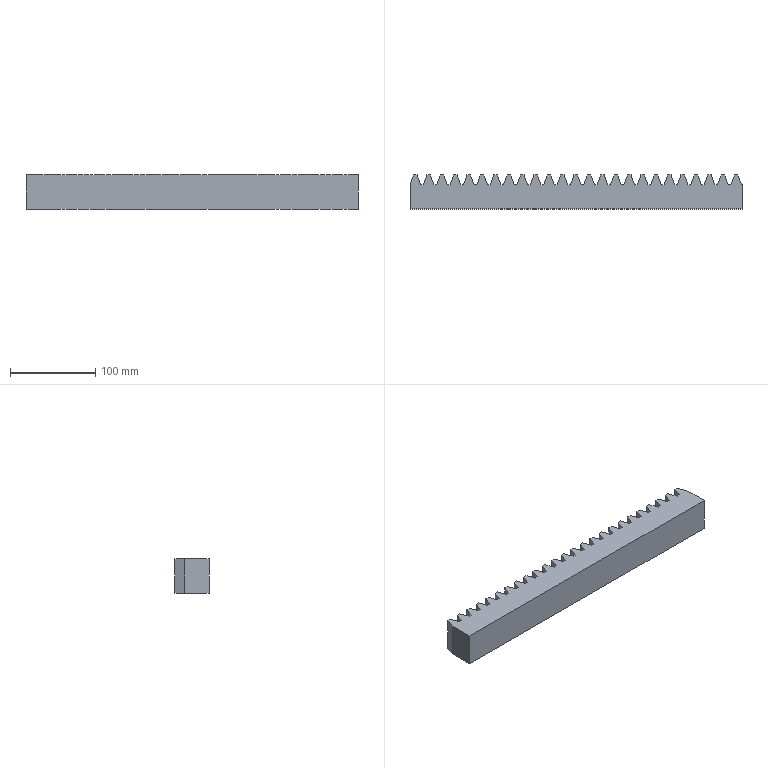Part | SolidWorks | features BaseBody 1 | 1 solid | 105 faces | box 390 x 40 x 40 mm | volume 541976 mm3 | plane 105